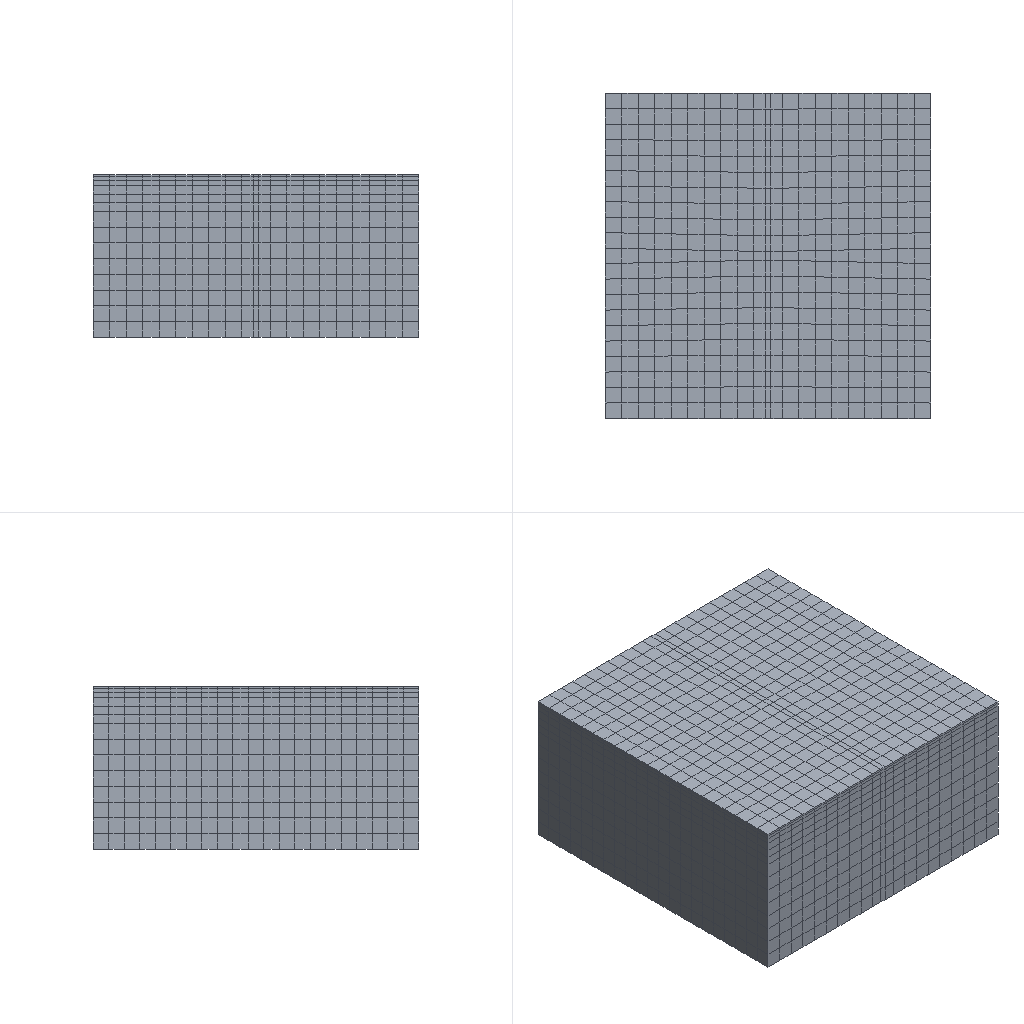Simulation study | abaqus
Set-up summary:
category,name,step,type,value,unit,region
solver,abaqus,,Abaqus/CAE 2024
units,SI m-kg-s (Pa),,inferred,E=6.544e+09 density=2390
analysis,Step-1,,heat transfer,time_period=86400
mesh,nodes,,,7260
mesh,elements,,,6174
element_type,DC3D8,,,6174
material,Material-1,,E,6.544e+09
material,Material-1,,nu,0.35
material,Material-1,,density,2390
material,Material-1,,conductivity,1.408
material,Material-1,,specific_heat,967
material,Material-1,,behaviors,conductivity; specific heat
material,Material-2,,E,1.0884e+10
material,Material-2,,nu,0.35
material,Material-2,,density,2430
material,Material-2,,conductivity,1.376
material,Material-2,,specific_heat,939
material,Material-2,,behaviors,conductivity; specific heat
material,Material-3,,E,8.652e+09
material,Material-3,,nu,0.35
material,Material-3,,density,1000
material,Material-3,,conductivity,0.5556
material,Material-3,,specific_heat,1430
material,Material-3,,behaviors,conductivity; specific heat
material,Material-4,,E,1.468e+09
material,Material-4,,nu,0.2
material,Material-4,,density,2300
material,Material-4,,conductivity,1.26
material,Material-4,,specific_heat,900
material,Material-4,,behaviors,conductivity; specific heat
material,Material-5,,E,5e+07
material,Material-5,,nu,0.35
material,Material-5,,density,1800
material,Material-5,,conductivity,0.86
material,Material-5,,specific_heat,800
material,Material-5,,behaviors,conductivity; specific heat
section,Material-5,,solid section,,,_PickedSet22
section,Material-4,,solid section,,,_PickedSet21
section,Material-3,,solid section,,,_PickedSet19
section,Material-2,,solid section,,,_PickedSet18
section,Material-1,,solid section,,,_PickedSet17
load,Predefined,initial,initial condition temperature
load,Int-1,Step-1,sfilm,0.9,,_PickedSurf9
load,Int-2,Step-1,sradiate,0.81,,_PickedSurf10
Abaqus input file, long lists of numbers shortened:
*Heading
** Job name: deck Model name: 0411
** Generated by: Abaqus/CAE 2024
*Preprint, echo=NO, model=NO, history=NO, contact=NO
**
** PARTS
**
*Part, name=lumian
*Node
      1, -0.4467,         0.25,   2.32
      2, -0.4467,        -5.75,   2.32
** (7258 more lines like these left out)
*Element, type=DC3D8
  1,    5,  159, 1537,  212,    1,  105, 1397,  158
  2,  159,  160, 1538, 1537,  105,  106, 1398, 1397
** (6172 more lines like these left out)
*Nset, nset=_PickedSet17, internal
   25,   26,   27,   28,   29,   30,   31,   32,   33,   34,   35,   36,   49,   50,   51,   52
   53,   54,   65,   66,   67,   68,   69,   70,   85,   86,   87,   88,   89,   90,  103,  104
** (59 more lines like these left out)
*Elset, elset=_PickedSet17, internal
  253,  254,  255,  256,  257,  258,  259,  260,  261,  262,  263,  264,  265,  266,  267,  268
  269,  270,  271,  272,  273,  526,  527,  528,  529,  530,  531,  532,  533,  534,  535,  536
** (26 more lines like these left out)
*Nset, nset=_PickedSet18, internal
   21,   22,   23,   24,   25,   26,   27,   28,   47,   48,   49,   50,   63,   64,   65,   66
   83,   84,   85,   86,   87,   90,   91,   92,  333,  334,  335,  336,  337,  338,  339,  340
** (59 more lines like these left out)
*Elset, elset=_PickedSet18, internal
  232,  233,  234,  235,  236,  237,  238,  239,  240,  241,  242,  243,  244,  245,  246,  247
  248,  249,  250,  251,  252,  505,  506,  507,  508,  509,  510,  511,  512,  513,  514,  515
** (26 more lines like these left out)
*Nset, nset=_PickedSet19, internal
   17,   18,   19,   20,   21,   22,   23,   24,   45,   46,   47,   48,   61,   62,   63,   64
   81,   82,   83,   84,   91,   92,   93,   94,  293,  294,  295,  296,  297,  298,  299,  300
** (59 more lines like these left out)
*Elset, elset=_PickedSet19, internal
  211,  212,  213,  214,  215,  216,  217,  218,  219,  220,  221,  222,  223,  224,  225,  226
  227,  228,  229,  230,  231,  484,  485,  486,  487,  488,  489,  490,  491,  492,  493,  494
** (26 more lines like these left out)
*Nset, nset=_PickedSet21, internal
    1,    2,    5,    6,    9,   10,   11,   12,   13,   14,   15,   16,   17,   18,   19,   20
   37,   38,   41,   42,   43,   44,   45,   46,   55,   56,   57,   58,   59,   60,   61,   62
** (119 more lines like these left out)
*Elset, elset=_PickedSet21, internal
  169,  170,  171,  172,  173,  174,  175,  176,  177,  178,  179,  180,  181,  182,  183,  184
  185,  186,  187,  188,  189,  190,  191,  192,  193,  194,  195,  196,  197,  198,  199,  200
** (81 more lines like these left out)
*Nset, nset=_PickedSet22, internal
    1,    2,    3,    4,    5,    6,    7,    8,   37,   38,   39,   40,   57,   58,   71,   72
   73,   74,   75,   76,   99,  100,  101,  102,  105,  106,  107,  108,  109,  110,  111,  112
** (271 more lines like these left out)
*Elset, elset=_PickedSet22, internal
    1,    2,    3,    4,    5,    6,    7,    8,    9,   10,   11,   12,   13,   14,   15,   16
   17,   18,   19,   20,   21,   22,   23,   24,   25,   26,   27,   28,   29,   30,   31,   32
** (219 more lines like these left out)
** Section: Section-5
*Solid Section, elset=_PickedSet22, material=Material-5
,
** Section: Section-4
*Solid Section, elset=_PickedSet21, material=Material-4
,
** Section: Section-3
*Solid Section, elset=_PickedSet19, material=Material-3
,
** Section: Section-2
*Solid Section, elset=_PickedSet18, material=Material-2
,
** Section: Section-1
*Solid Section, elset=_PickedSet17, material=Material-1
,
*End Part
**
**
** ASSEMBLY
**
*Assembly, name=Assembly
**
*Instance, name=lumian-1, part=lumian
*End Instance
**
*Nset, nset=_PickedSet8, internal, instance=lumian-1, generate
    1,  7260,     1
*Elset, elset=_PickedSet8, internal, instance=lumian-1, generate
    1,  6174,     1
*Elset, elset=__PickedSurf9_S6, internal, instance=lumian-1
 253, 254, 255, 256, 257, 258, 259, 260, 261, 262, 263, 264, 265, 266, 267, 268
 269, 270, 271, 272, 273, 526, 527, 528, 529, 530, 531, 532, 533, 534, 535, 536
** (2 more lines like these left out)
*Elset, elset=__PickedSurf9_S1, internal, instance=lumian-1, generate
 5797,  5985,     1
*Elset, elset=__PickedSurf9_S5, internal, instance=lumian-1, generate
 3340,  3528,     1
*Surface, type=ELEMENT, name=_PickedSurf9, internal
__PickedSurf9_S6, S6
__PickedSurf9_S1, S1
__PickedSurf9_S5, S5
*Elset, elset=__PickedSurf10_S6, internal, instance=lumian-1
 253, 254, 255, 256, 257, 258, 259, 260, 261, 262, 263, 264, 265, 266, 267, 268
 269, 270, 271, 272, 273, 526, 527, 528, 529, 530, 531, 532, 533, 534, 535, 536
** (2 more lines like these left out)
*Elset, elset=__PickedSurf10_S1, internal, instance=lumian-1, generate
 5797,  5985,     1
*Elset, elset=__PickedSurf10_S5, internal, instance=lumian-1, generate
 3340,  3528,     1
*Surface, type=ELEMENT, name=_PickedSurf10, internal
__PickedSurf10_S6, S6
__PickedSurf10_S1, S1
__PickedSurf10_S5, S5
*End Assembly
*Amplitude, name=Amp-CHUN
          3600.,             5.7,           7200.,             3.7,          10800.,             3.3,          14400.,             2.6
         18000.,              2.,          21600.,             0.3,          25200.,             0.3,          28800.,             1.2
         32400.,             4.2,          36000.,             8.9,          39600.,            13.2,          43200.,            17.3
         46800.,            18.9,          50400.,            21.1,          54000.,            22.6,          57600.,            22.3
         61200.,            22.4,          64800.,            21.4,          68400.,            18.1,          72000.,            15.9
         75600.,            14.2,          79200.,            11.3,          82800.,            12.8,          86400.,             9.2
*Amplitude, name=Amp-DONG
          3600.,            -5.2,           7200.,            -5.2,          10800.,            -5.4,          14400.,            -5.4
         18000.,            -5.5,          21600.,            -5.5,          25200.,            -5.6,          28800.,            -5.6
         32400.,            -5.3,          36000.,            -4.6,          39600.,            -3.3,          43200.,            -1.6
         46800.,            -0.5,          50400.,            -0.2,          54000.,            -0.1,          57600.,            -0.2
         61200.,            -0.8,          64800.,            -2.1,          68400.,            -3.7,          72000.,            -3.9
         75600.,            -4.1,          79200.,            -4.2,          82800.,            -3.9,          86400.,            -3.5
*Amplitude, name=Amp-QIU
          3600.,             24.,           7200.,            22.5,          10800.,            21.9,          14400.,            21.6
         18000.,            20.9,          21600.,             21.,          25200.,            21.1,          28800.,            22.7
         32400.,            24.6,          36000.,             27.,          39600.,            28.9,          43200.,            30.5
         46800.,            31.8,          50400.,            32.8,          54000.,            33.3,          57600.,            33.7
         61200.,            33.2,          64800.,            32.5,          68400.,            31.2,          72000.,            29.5
         75600.,             29.,          79200.,            28.2,          82800.,            27.5,          86400.,             27.
*Amplitude, name=Amp-XIA
          3600.,            12.2,           7200.,            11.2,          10800.,            10.6,          14400.,             9.5
         18000.,             8.9,          21600.,             8.8,          25200.,             8.9,          28800.,            10.3
         32400.,            12.8,          36000.,            15.4,          39600.,            17.5,          43200.,            19.1
         46800.,            20.3,          50400.,            21.1,          54000.,            21.8,          57600.,            22.1
         61200.,             22.,          64800.,            20.8,          68400.,            17.5,          72000.,            15.9
         75600.,            15.2,          79200.,            15.5,          82800.,            14.6,          86400.,            13.6
**
** MATERIALS
**
*Material, name=Material-1
*Conductivity
 1.408,
*Density
2390.,
*Elastic
 6.544e+09, 0.35
*Specific Heat
967.,
*Material, name=Material-2
*Conductivity
 1.376,
*Density
2430.,
*Elastic
 1.0884e+10, 0.35
*Specific Heat
939.,
*Material, name=Material-3
*Conductivity
 0.5556,
*Density
1000.,
*Elastic
 8.652e+09, 0.35
*Specific Heat
1430.,
*Material, name=Material-4
*Conductivity
 1.26,
*Density
2300.,
*Elastic
 1.468e+09, 0.2
*Specific Heat
900.,
*Material, name=Material-5
*Conductivity
 0.86,
*Density
1800.,
*Elastic
 5e+07, 0.35
*Specific Heat
800.,
**
** PHYSICAL CONSTANTS
**
*Physical Constants, absolute zero=-273., stefan boltzmann=5.67e-08
**
** PREDEFINED FIELDS
**
** Name: Predefined Field-1   Type: Temperature
*Initial Conditions, type=TEMPERATURE
_PickedSet8, 13.2
** ----------------------------------------------------------------
**
** STEP: Step-1
**
*Step, name=Step-1, nlgeom=NO, inc=10000
*Heat Transfer, end=PERIOD, deltmx=50.
360., 86400., 0.864, 1800.,
**
** INTERACTIONS
**
** Interaction: Int-1
*Sfilm, amplitude=Amp-CHUN
_PickedSurf9, F, 1., 0.9
** Interaction: Int-2
*Sradiate, amplitude=Amp-CHUN
_PickedSurf10, R, 1., 0.81
**
** OUTPUT REQUESTS
**
*Restart, write, frequency=0
**
** FIELD OUTPUT: F-Output-1
**
*Output, field, number interval=48
*Node Output
NT, RFL
*Element Output, directions=YES
HFL, TEMP
*Output, history, frequency=0
*End Step
Results summary:
result,odb.job_status,,,JOB_STATUS_COMPLETED_SUCCESSFULLY,"consistent, unstated (Abaqus has no unit system)"
result,steps[0].procedure,Step-1,,"*HEAT TRANSFER, DELTAMX","consistent, unstated (Abaqus has no unit system)"
result,steps[0].time_period,Step-1,,86400,"consistent, unstated (Abaqus has no unit system)"
result,steps[0].n_frames,Step-1,,49,"consistent, unstated (Abaqus has no unit system)"
result,steps[0].last_frame.id,Step-1,,51,"consistent, unstated (Abaqus has no unit system)"
result,steps[0].last_frame.value,Step-1,,86400,"consistent, unstated (Abaqus has no unit system)"
result,steps[0].last_frame.description,Step-1,,Increment     51: Step Time =   8.6400E+04,"consistent, unstated (Abaqus has no unit system)"
result,steps[0].completed,Step-1,,True,"consistent, unstated (Abaqus has no unit system)"